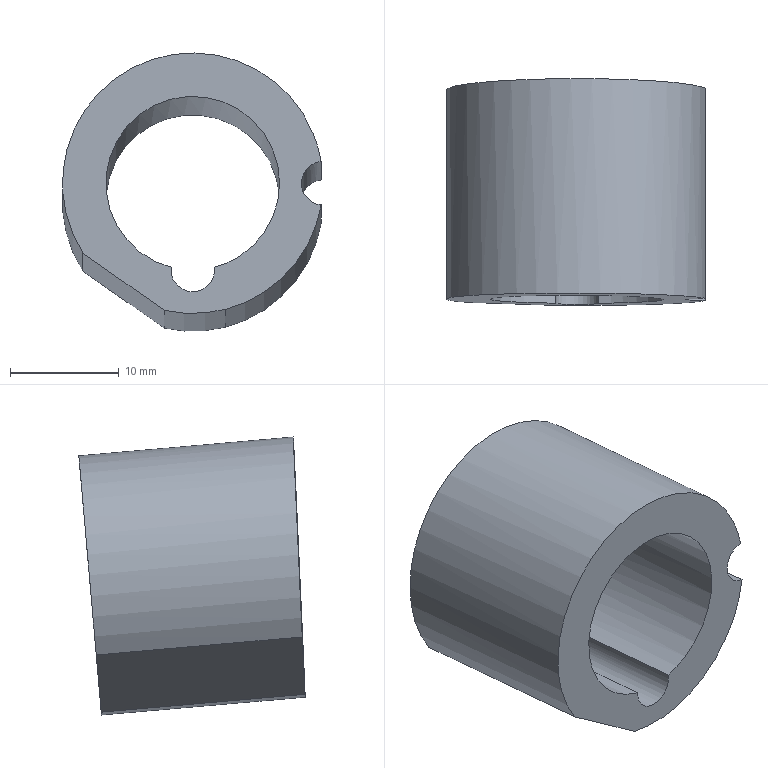Part | NX | features solid 2 | 1 solid | 9 faces | box 23.833 x 20.851 x 25.637 mm | volume 4510 mm3 | cylinder 5 | plane 3 | spline 1 | commonest cylinder face diameters 4 x2 24 x2 16 x1
STEP:
#1=CARTESIAN_POINT('',(159.152,-46.323,-37.666));
#2=VERTEX_POINT('',#1);
#3=CARTESIAN_POINT('',(159.152,-27.352,-39.326));
#4=VERTEX_POINT('',#3);
#5=CARTESIAN_POINT('',(159.152,-27.352,-39.326));
#6=DIRECTION('',(0.,-0.9962,0.08716));
#7=VECTOR('',#6,1000.);
#8=LINE('',#5,#7);
#9=EDGE_CURVE('',#2,#4,#8,.F.);
#10=ORIENTED_EDGE('',*,*,#9,.F.);
#11=CARTESIAN_POINT('',(181.121,-45.983,-29.247));
#12=VERTEX_POINT('',#11);
#13=CARTESIAN_POINT('',(169.288,-46.051,-31.241));
#14=DIRECTION('',(0.001957,0.999,-0.04546));
#15=DIRECTION('',(0.04675,0.04532,0.9979));
#16=AXIS2_PLACEMENT_3D('',#13,#14,#15);
#17=ELLIPSE('',#16,12.011,12.);
#18=EDGE_CURVE('',#2,#12,#17,.T.);
#19=ORIENTED_EDGE('',*,*,#18,.T.);
#20=CARTESIAN_POINT('',(181.121,-26.618,-30.941));
#21=VERTEX_POINT('',#20);
#22=CARTESIAN_POINT('',(181.121,-36.359,-30.089));
#23=DIRECTION('',(0.,0.9962,-0.08716));
#24=VECTOR('',#23,1000.);
#25=LINE('',#22,#24);
#26=EDGE_CURVE('',#12,#21,#25,.T.);
#27=ORIENTED_EDGE('',*,*,#26,.T.);
#28=CARTESIAN_POINT('',(169.288,-26.792,-32.926));
#29=DIRECTION('',(0.,0.9962,-0.08716));
#30=DIRECTION('',(0.,-0.08716,-0.9962));
#31=AXIS2_PLACEMENT_3D('',#28,#29,#30);
#32=CIRCLE('',#31,12.);
#33=EDGE_CURVE('',#4,#21,#32,.T.);
#34=ORIENTED_EDGE('',*,*,#33,.F.);
#35=EDGE_LOOP('',(#10,#19,#27,#34));
#36=FACE_BOUND('',#35,.T.);
#37=CARTESIAN_POINT('',(169.288,-26.792,-32.926));
#38=DIRECTION('',(0.,-0.9962,0.08716));
#39=DIRECTION('',(0.,-0.08716,-0.9962));
#40=AXIS2_PLACEMENT_3D('',#37,#38,#39);
#41=CYLINDRICAL_SURFACE('',#40,12.);
#42=ADVANCED_FACE('',(#36),#41,.T.);
#43=CARTESIAN_POINT('',(167.304,-46.399,-38.991));
#44=VERTEX_POINT('',#43);
#45=CARTESIAN_POINT('',(171.272,-46.407,-38.99));
#46=VERTEX_POINT('',#45);
#47=CARTESIAN_POINT('',(169.288,-46.051,-31.241));
#48=DIRECTION('',(0.001957,0.999,-0.04546));
#49=DIRECTION('',(0.04675,0.04532,0.9979));
#50=AXIS2_PLACEMENT_3D('',#47,#48,#49);
#51=ELLIPSE('',#50,8.007,8.);
#52=EDGE_CURVE('',#44,#46,#51,.T.);
#53=ORIENTED_EDGE('',*,*,#52,.T.);
#54=CARTESIAN_POINT('',(169.288,-46.415,-39.24));
#55=DIRECTION('',(0.001957,0.999,-0.04546));
#56=DIRECTION('',(-0.04675,-0.04532,-0.9979));
#57=AXIS2_PLACEMENT_3D('',#54,#55,#56);
#58=ELLIPSE('',#57,2.002,2.);
#59=EDGE_CURVE('',#46,#44,#58,.T.);
#60=ORIENTED_EDGE('',*,*,#59,.T.);
#61=EDGE_LOOP('',(#53,#60));
#62=FACE_BOUND('',#61,.T.);
#63=CARTESIAN_POINT('',(166.66,-46.578,-42.949));
#64=VERTEX_POINT('',#63);
#65=CARTESIAN_POINT('',(162.955,-46.452,-40.342));
#66=DIRECTION('',(-0.8175,0.02778,0.5752));
#67=VECTOR('',#66,1000.);
#68=LINE('',#65,#67);
#69=EDGE_CURVE('',#64,#2,#68,.T.);
#70=ORIENTED_EDGE('',*,*,#69,.F.);
#71=CARTESIAN_POINT('',(172.264,-46.585,-42.864));
#72=VERTEX_POINT('',#71);
#73=CARTESIAN_POINT('',(166.66,-46.578,-42.949));
#74=CARTESIAN_POINT('',(168.503,-46.601,-43.362));
#75=CARTESIAN_POINT('',(170.431,-46.603,-43.334));
#76=CARTESIAN_POINT('',(172.264,-46.585,-42.864));
#77=B_SPLINE_CURVE_WITH_KNOTS('',3,(#73,#74,#75,#76),.UNSPECIFIED.,.F.,.F.,(4,4),(0.0003576,0.006022),.UNSPECIFIED.);
#78=EDGE_CURVE('',#64,#72,#77,.T.);
#79=ORIENTED_EDGE('',*,*,#78,.T.);
#80=CARTESIAN_POINT('',(181.121,-46.164,-33.232));
#81=VERTEX_POINT('',#80);
#82=CARTESIAN_POINT('',(169.288,-46.051,-31.241));
#83=DIRECTION('',(0.001957,0.999,-0.04546));
#84=DIRECTION('',(0.04675,0.04532,0.9979));
#85=AXIS2_PLACEMENT_3D('',#82,#83,#84);
#86=ELLIPSE('',#85,12.011,12.);
#87=EDGE_CURVE('',#81,#72,#86,.T.);
#88=ORIENTED_EDGE('',*,*,#87,.F.);
#89=CARTESIAN_POINT('',(181.288,-46.074,-31.239));
#90=DIRECTION('',(0.001957,0.999,-0.04546));
#91=DIRECTION('',(-0.04675,-0.04532,-0.9979));
#92=AXIS2_PLACEMENT_3D('',#89,#90,#91);
#93=ELLIPSE('',#92,2.002,2.);
#94=EDGE_CURVE('',#81,#12,#93,.T.);
#95=ORIENTED_EDGE('',*,*,#94,.T.);
#96=ORIENTED_EDGE('',*,*,#18,.F.);
#97=EDGE_LOOP('',(#70,#79,#88,#95,#96));
#98=FACE_BOUND('',#97,.T.);
#99=CARTESIAN_POINT('',(128.811,-48.589,-88.763));
#100=DIRECTION('',(0.001957,0.999,-0.04546));
#101=DIRECTION('',(0.06617,0.04523,0.9968));
#102=AXIS2_PLACEMENT_3D('',#99,#100,#101);
#103=PLANE('',#102);
#104=ADVANCED_FACE('',(#62,#98),#103,.F.);
#105=CARTESIAN_POINT('',(167.304,-27.467,-40.647));
#106=VERTEX_POINT('',#105);
#107=CARTESIAN_POINT('',(171.272,-27.467,-40.647));
#108=VERTEX_POINT('',#107);
#109=CARTESIAN_POINT('',(169.288,-26.792,-32.926));
#110=DIRECTION('',(0.,-0.9962,0.08716));
#111=DIRECTION('',(0.,-0.08716,-0.9962));
#112=AXIS2_PLACEMENT_3D('',#109,#110,#111);
#113=CIRCLE('',#112,8.);
#114=EDGE_CURVE('',#106,#108,#113,.F.);
#115=ORIENTED_EDGE('',*,*,#114,.F.);
#116=CARTESIAN_POINT('',(169.288,-27.489,-40.896));
#117=DIRECTION('',(0.,-0.9962,0.08716));
#118=DIRECTION('',(0.,0.08716,0.9962));
#119=AXIS2_PLACEMENT_3D('',#116,#117,#118);
#120=CIRCLE('',#119,2.);
#121=EDGE_CURVE('',#106,#108,#120,.T.);
#122=ORIENTED_EDGE('',*,*,#121,.T.);
#123=EDGE_LOOP('',(#115,#122));
#124=FACE_BOUND('',#123,.T.);
#125=CARTESIAN_POINT('',(166.66,-27.812,-44.59));
#126=VERTEX_POINT('',#125);
#127=CARTESIAN_POINT('',(166.387,-27.796,-44.4));
#128=DIRECTION('',(-0.8177,0.05017,0.5734));
#129=VECTOR('',#128,1000.);
#130=LINE('',#127,#129);
#131=EDGE_CURVE('',#4,#126,#130,.F.);
#132=ORIENTED_EDGE('',*,*,#131,.F.);
#133=ORIENTED_EDGE('',*,*,#33,.T.);
#134=CARTESIAN_POINT('',(181.121,-26.966,-34.912));
#135=VERTEX_POINT('',#134);
#136=CARTESIAN_POINT('',(181.288,-26.792,-32.926));
#137=DIRECTION('',(0.,-0.9962,0.08716));
#138=DIRECTION('',(0.,0.08716,0.9962));
#139=AXIS2_PLACEMENT_3D('',#136,#137,#138);
#140=CIRCLE('',#139,2.);
#141=EDGE_CURVE('',#21,#135,#140,.T.);
#142=ORIENTED_EDGE('',*,*,#141,.T.);
#143=CARTESIAN_POINT('',(172.264,-27.805,-44.507));
#144=VERTEX_POINT('',#143);
#145=CARTESIAN_POINT('',(169.288,-26.792,-32.926));
#146=DIRECTION('',(0.,0.9962,-0.08716));
#147=DIRECTION('',(0.,-0.08716,-0.9962));
#148=AXIS2_PLACEMENT_3D('',#145,#146,#147);
#149=CIRCLE('',#148,12.);
#150=EDGE_CURVE('',#135,#144,#149,.T.);
#151=ORIENTED_EDGE('',*,*,#150,.T.);
#152=CARTESIAN_POINT('',(166.311,-27.805,-44.507));
#153=CARTESIAN_POINT('',(168.264,-27.849,-45.005));
#154=CARTESIAN_POINT('',(170.311,-27.849,-45.005));
#155=CARTESIAN_POINT('',(172.264,-27.805,-44.507));
#156=B_SPLINE_CURVE_WITH_KNOTS('',3,(#152,#153,#154,#155),.UNSPECIFIED.,.F.,.F.,(4,4),(0.,1.),.PIECEWISE_BEZIER_KNOTS.);
#157=EDGE_CURVE('',#126,#144,#156,.T.);
#158=ORIENTED_EDGE('',*,*,#157,.F.);
#159=EDGE_LOOP('',(#132,#133,#142,#151,#158));
#160=FACE_BOUND('',#159,.T.);
#161=CARTESIAN_POINT('',(166.311,-27.805,-44.507));
#162=DIRECTION('',(0.,0.9962,-0.08716));
#163=DIRECTION('',(0.,0.08716,0.9962));
#164=AXIS2_PLACEMENT_3D('',#161,#162,#163);
#165=PLANE('',#164);
#166=ADVANCED_FACE('',(#124,#160),#165,.T.);
#167=ORIENTED_EDGE('',*,*,#78,.F.);
#168=CARTESIAN_POINT('',(166.66,-27.812,-44.59));
#169=DIRECTION('',(0.,-0.9962,0.08716));
#170=VECTOR('',#169,1000.);
#171=LINE('',#168,#170);
#172=EDGE_CURVE('',#64,#126,#171,.F.);
#173=ORIENTED_EDGE('',*,*,#172,.T.);
#174=ORIENTED_EDGE('',*,*,#157,.T.);
#175=CARTESIAN_POINT('',(172.264,-27.805,-44.507));
#176=DIRECTION('',(0.,-0.9962,0.08716));
#177=VECTOR('',#176,1000.);
#178=LINE('',#175,#177);
#179=EDGE_CURVE('',#144,#72,#178,.T.);
#180=ORIENTED_EDGE('',*,*,#179,.T.);
#181=EDGE_LOOP('',(#167,#173,#174,#180));
#182=FACE_BOUND('',#181,.T.);
#183=CARTESIAN_POINT('',(166.66,-27.812,-44.59));
#184=CARTESIAN_POINT('',(166.66,-46.705,-42.938));
#185=CARTESIAN_POINT('',(168.507,-27.848,-45.004));
#186=CARTESIAN_POINT('',(168.507,-46.741,-43.351));
#187=CARTESIAN_POINT('',(170.427,-27.846,-44.976));
#188=CARTESIAN_POINT('',(170.427,-46.739,-43.323));
#189=CARTESIAN_POINT('',(172.264,-27.805,-44.507));
#190=CARTESIAN_POINT('',(172.264,-46.698,-42.854));
#191=B_SPLINE_SURFACE_WITH_KNOTS('',3,1,((#183,#184),(#185,#186),(#187,#188),(#189,#190)),.SURF_OF_LINEAR_EXTRUSION.,.F.,.F.,.F.,(4,4),(2,2),(0.05926,1.),(0.,1.),.PIECEWISE_BEZIER_KNOTS.);
#192=ADVANCED_FACE('',(#182),#191,.T.);
#193=ORIENTED_EDGE('',*,*,#52,.F.);
#194=CARTESIAN_POINT('',(167.304,-27.467,-40.647));
#195=DIRECTION('',(0.,-0.9962,0.08716));
#196=VECTOR('',#195,1000.);
#197=LINE('',#194,#196);
#198=EDGE_CURVE('',#106,#44,#197,.T.);
#199=ORIENTED_EDGE('',*,*,#198,.F.);
#200=ORIENTED_EDGE('',*,*,#114,.T.);
#201=CARTESIAN_POINT('',(171.272,-27.467,-40.647));
#202=DIRECTION('',(0.,-0.9962,0.08716));
#203=VECTOR('',#202,1000.);
#204=LINE('',#201,#203);
#205=EDGE_CURVE('',#46,#108,#204,.F.);
#206=ORIENTED_EDGE('',*,*,#205,.F.);
#207=EDGE_LOOP('',(#193,#199,#200,#206));
#208=FACE_BOUND('',#207,.T.);
#209=CARTESIAN_POINT('',(169.288,-26.792,-32.926));
#210=DIRECTION('',(0.,-0.9962,0.08716));
#211=DIRECTION('',(0.,-0.08716,-0.9962));
#212=AXIS2_PLACEMENT_3D('',#209,#210,#211);
#213=CYLINDRICAL_SURFACE('',#212,8.);
#214=ADVANCED_FACE('',(#208),#213,.F.);
#215=ORIENTED_EDGE('',*,*,#150,.F.);
#216=CARTESIAN_POINT('',(181.121,-36.706,-34.06));
#217=DIRECTION('',(0.,0.9962,-0.08716));
#218=VECTOR('',#217,1000.);
#219=LINE('',#216,#218);
#220=EDGE_CURVE('',#135,#81,#219,.F.);
#221=ORIENTED_EDGE('',*,*,#220,.T.);
#222=ORIENTED_EDGE('',*,*,#87,.T.);
#223=ORIENTED_EDGE('',*,*,#179,.F.);
#224=EDGE_LOOP('',(#215,#221,#222,#223));
#225=FACE_BOUND('',#224,.T.);
#226=CARTESIAN_POINT('',(169.288,-26.792,-32.926));
#227=DIRECTION('',(0.,-0.9962,0.08716));
#228=DIRECTION('',(0.,-0.08716,-0.9962));
#229=AXIS2_PLACEMENT_3D('',#226,#227,#228);
#230=CYLINDRICAL_SURFACE('',#229,12.);
#231=ADVANCED_FACE('',(#225),#230,.T.);
#232=ORIENTED_EDGE('',*,*,#59,.F.);
#233=ORIENTED_EDGE('',*,*,#205,.T.);
#234=ORIENTED_EDGE('',*,*,#121,.F.);
#235=ORIENTED_EDGE('',*,*,#198,.T.);
#236=EDGE_LOOP('',(#232,#233,#234,#235));
#237=FACE_BOUND('',#236,.T.);
#238=CARTESIAN_POINT('',(169.288,-47.413,-39.153));
#239=DIRECTION('',(0.,0.9962,-0.08716));
#240=DIRECTION('',(0.,-0.08716,-0.9962));
#241=AXIS2_PLACEMENT_3D('',#238,#239,#240);
#242=CYLINDRICAL_SURFACE('',#241,2.);
#243=ADVANCED_FACE('',(#237),#242,.F.);
#244=ORIENTED_EDGE('',*,*,#94,.F.);
#245=ORIENTED_EDGE('',*,*,#220,.F.);
#246=ORIENTED_EDGE('',*,*,#141,.F.);
#247=ORIENTED_EDGE('',*,*,#26,.F.);
#248=EDGE_LOOP('',(#244,#245,#246,#247));
#249=FACE_BOUND('',#248,.T.);
#250=CARTESIAN_POINT('',(181.288,-46.716,-31.183));
#251=DIRECTION('',(0.,0.9962,-0.08716));
#252=DIRECTION('',(0.,-0.08716,-0.9962));
#253=AXIS2_PLACEMENT_3D('',#250,#251,#252);
#254=CYLINDRICAL_SURFACE('',#253,2.);
#255=ADVANCED_FACE('',(#249),#254,.F.);
#256=ORIENTED_EDGE('',*,*,#69,.T.);
#257=ORIENTED_EDGE('',*,*,#9,.T.);
#258=ORIENTED_EDGE('',*,*,#131,.T.);
#259=ORIENTED_EDGE('',*,*,#172,.F.);
#260=EDGE_LOOP('',(#256,#257,#258,#259));
#261=FACE_BOUND('',#260,.T.);
#262=CARTESIAN_POINT('',(159.152,53.296,-46.381));
#263=DIRECTION('',(-0.5756,-0.07127,-0.8146));
#264=DIRECTION('',(-0.8167,0.,0.5771));
#265=AXIS2_PLACEMENT_3D('',#262,#263,#264);
#266=PLANE('',#265);
#267=ADVANCED_FACE('',(#261),#266,.T.);
#268=CLOSED_SHELL('',(#42,#104,#166,#192,#214,#231,#243,#255,#267));
#269=MANIFOLD_SOLID_BREP('',#268);
#270=(LENGTH_UNIT()NAMED_UNIT(*)SI_UNIT(.MILLI.,.METRE.));
#271=UNCERTAINTY_MEASURE_WITH_UNIT(LENGTH_MEASURE(0.0508),#270,'','');
#272=(NAMED_UNIT(*)PLANE_ANGLE_UNIT()SI_UNIT($,.RADIAN.));
#273=(NAMED_UNIT(*)SI_UNIT($,.STERADIAN.)SOLID_ANGLE_UNIT());
#274=(GEOMETRIC_REPRESENTATION_CONTEXT(3)GLOBAL_UNCERTAINTY_ASSIGNED_CONTEXT((#271))GLOBAL_UNIT_ASSIGNED_CONTEXT((#270,#272,#273))REPRESENTATION_CONTEXT('',''));
#275=ADVANCED_BREP_SHAPE_REPRESENTATION('',(#269),#274);